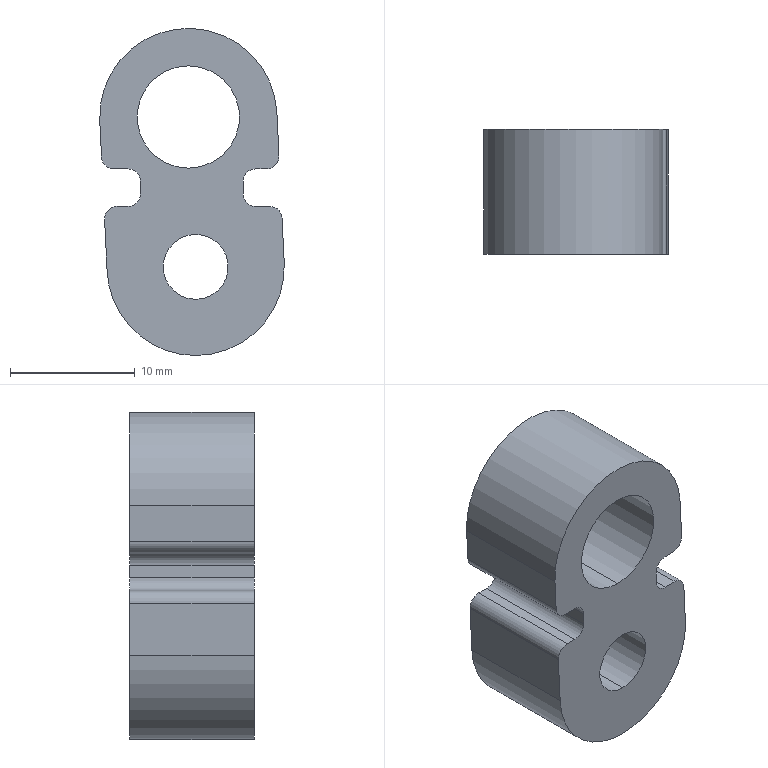Part | STEP file | Rotating slot | 1 solid | 27 faces | box 14.79 x 10 x 26.2 mm | volume 2369 mm3 | cylinder 15 | plane 12 | commonest cylinder face diameters 2 x8 14.2 x3 5.2 x2 8.2 x2